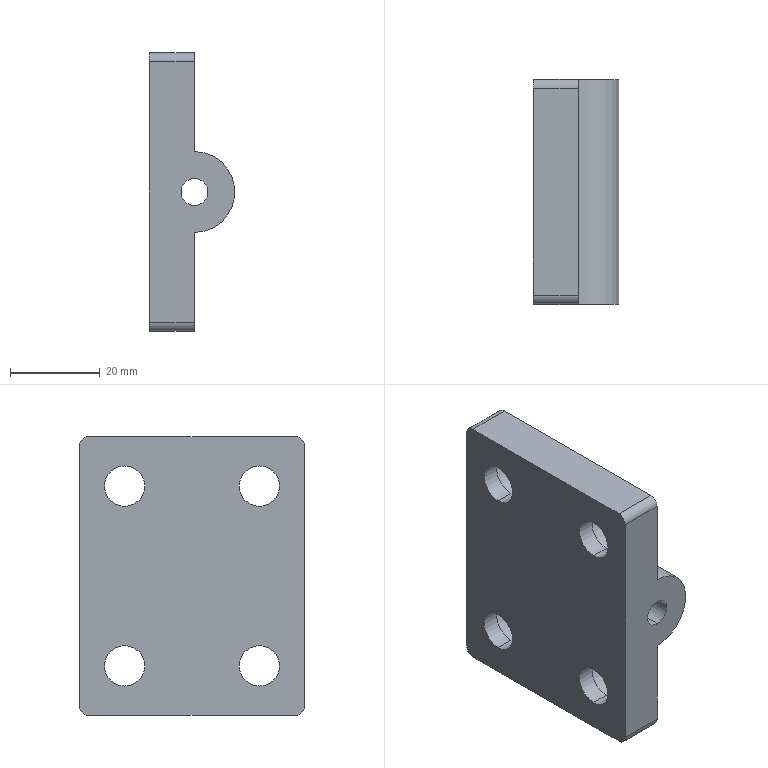Part | SolidWorks | features Extrusion 1, Fillet 1, HoleWzd 1 | 1 solid | 34 faces | box 19 x 50 x 62 mm | volume 31201 mm3 | cylinder 23 | plane 11 | commonest cylinder face diameters 9 x8 14 x8 4 x4 6 x2 18 x1
STEP:
#1=CARTESIAN_POINT('',(4.,15.,27.));
#2=VERTEX_POINT('',#1);
#3=CARTESIAN_POINT('',(4.,15.,13.));
#4=VERTEX_POINT('',#3);
#5=CARTESIAN_POINT('',(4.,15.,20.));
#6=DIRECTION('',(1.,0.,0.));
#7=DIRECTION('',(0.,0.,-1.));
#8=AXIS2_PLACEMENT_3D('',#5,#6,#7);
#9=CIRCLE('',#8,7.);
#10=EDGE_CURVE('',#2,#4,#9,.T.);
#11=ORIENTED_EDGE('',*,*,#10,.F.);
#12=CARTESIAN_POINT('',(10.,15.,27.));
#13=VERTEX_POINT('',#12);
#14=CARTESIAN_POINT('',(10.,15.,27.));
#15=DIRECTION('',(1.,0.,0.));
#16=VECTOR('',#15,1000.);
#17=LINE('',#14,#16);
#18=EDGE_CURVE('',#2,#13,#17,.T.);
#19=ORIENTED_EDGE('',*,*,#18,.T.);
#20=CARTESIAN_POINT('',(10.,15.,13.));
#21=VERTEX_POINT('',#20);
#22=CARTESIAN_POINT('',(10.,15.,20.));
#23=DIRECTION('',(1.,0.,0.));
#24=DIRECTION('',(0.,0.,-1.));
#25=AXIS2_PLACEMENT_3D('',#22,#23,#24);
#26=CIRCLE('',#25,7.);
#27=EDGE_CURVE('',#13,#21,#26,.T.);
#28=ORIENTED_EDGE('',*,*,#27,.T.);
#29=CARTESIAN_POINT('',(10.,15.,13.));
#30=DIRECTION('',(1.,0.,0.));
#31=VECTOR('',#30,1000.);
#32=LINE('',#29,#31);
#33=EDGE_CURVE('',#4,#21,#32,.T.);
#34=ORIENTED_EDGE('',*,*,#33,.F.);
#35=EDGE_LOOP('',(#11,#19,#28,#34));
#36=FACE_OUTER_BOUND('',#35,.T.);
#37=CARTESIAN_POINT('',(10.,15.,20.));
#38=DIRECTION('',(1.,0.,0.));
#39=DIRECTION('',(0.,0.,-1.));
#40=AXIS2_PLACEMENT_3D('',#37,#38,#39);
#41=CYLINDRICAL_SURFACE('',#40,7.);
#42=ADVANCED_FACE('',(#36),#41,.F.);
#43=CARTESIAN_POINT('',(0.,15.,24.5));
#44=VERTEX_POINT('',#43);
#45=CARTESIAN_POINT('',(0.,15.,15.5));
#46=VERTEX_POINT('',#45);
#47=CARTESIAN_POINT('',(0.,15.,20.));
#48=DIRECTION('',(1.,0.,0.));
#49=DIRECTION('',(0.,0.,-1.));
#50=AXIS2_PLACEMENT_3D('',#47,#48,#49);
#51=CIRCLE('',#50,4.5);
#52=EDGE_CURVE('',#44,#46,#51,.T.);
#53=ORIENTED_EDGE('',*,*,#52,.F.);
#54=CARTESIAN_POINT('',(4.,15.,24.5));
#55=VERTEX_POINT('',#54);
#56=CARTESIAN_POINT('',(10.,15.,24.5));
#57=DIRECTION('',(1.,0.,0.));
#58=VECTOR('',#57,1000.);
#59=LINE('',#56,#58);
#60=EDGE_CURVE('',#44,#55,#59,.T.);
#61=ORIENTED_EDGE('',*,*,#60,.T.);
#62=CARTESIAN_POINT('',(4.,15.,15.5));
#63=VERTEX_POINT('',#62);
#64=CARTESIAN_POINT('',(4.,15.,20.));
#65=DIRECTION('',(1.,0.,0.));
#66=DIRECTION('',(0.,0.,-1.));
#67=AXIS2_PLACEMENT_3D('',#64,#65,#66);
#68=CIRCLE('',#67,4.5);
#69=EDGE_CURVE('',#55,#63,#68,.T.);
#70=ORIENTED_EDGE('',*,*,#69,.T.);
#71=CARTESIAN_POINT('',(10.,15.,15.5));
#72=DIRECTION('',(1.,0.,0.));
#73=VECTOR('',#72,1000.);
#74=LINE('',#71,#73);
#75=EDGE_CURVE('',#46,#63,#74,.T.);
#76=ORIENTED_EDGE('',*,*,#75,.F.);
#77=EDGE_LOOP('',(#53,#61,#70,#76));
#78=FACE_OUTER_BOUND('',#77,.T.);
#79=CARTESIAN_POINT('',(10.,15.,20.));
#80=DIRECTION('',(1.,0.,0.));
#81=DIRECTION('',(0.,0.,-1.));
#82=AXIS2_PLACEMENT_3D('',#79,#80,#81);
#83=CYLINDRICAL_SURFACE('',#82,4.5);
#84=ADVANCED_FACE('',(#78),#83,.F.);
#85=CARTESIAN_POINT('',(4.,-15.,27.));
#86=VERTEX_POINT('',#85);
#87=CARTESIAN_POINT('',(4.,-15.,13.));
#88=VERTEX_POINT('',#87);
#89=CARTESIAN_POINT('',(4.,-15.,20.));
#90=DIRECTION('',(1.,0.,0.));
#91=DIRECTION('',(0.,0.,-1.));
#92=AXIS2_PLACEMENT_3D('',#89,#90,#91);
#93=CIRCLE('',#92,7.);
#94=EDGE_CURVE('',#86,#88,#93,.T.);
#95=ORIENTED_EDGE('',*,*,#94,.F.);
#96=CARTESIAN_POINT('',(10.,-15.,27.));
#97=VERTEX_POINT('',#96);
#98=CARTESIAN_POINT('',(10.,-15.,27.));
#99=DIRECTION('',(1.,0.,0.));
#100=VECTOR('',#99,1000.);
#101=LINE('',#98,#100);
#102=EDGE_CURVE('',#86,#97,#101,.T.);
#103=ORIENTED_EDGE('',*,*,#102,.T.);
#104=CARTESIAN_POINT('',(10.,-15.,13.));
#105=VERTEX_POINT('',#104);
#106=CARTESIAN_POINT('',(10.,-15.,20.));
#107=DIRECTION('',(1.,0.,0.));
#108=DIRECTION('',(0.,0.,-1.));
#109=AXIS2_PLACEMENT_3D('',#106,#107,#108);
#110=CIRCLE('',#109,7.);
#111=EDGE_CURVE('',#97,#105,#110,.T.);
#112=ORIENTED_EDGE('',*,*,#111,.T.);
#113=CARTESIAN_POINT('',(10.,-15.,13.));
#114=DIRECTION('',(1.,0.,0.));
#115=VECTOR('',#114,1000.);
#116=LINE('',#113,#115);
#117=EDGE_CURVE('',#88,#105,#116,.T.);
#118=ORIENTED_EDGE('',*,*,#117,.F.);
#119=EDGE_LOOP('',(#95,#103,#112,#118));
#120=FACE_OUTER_BOUND('',#119,.T.);
#121=CARTESIAN_POINT('',(10.,-15.,20.));
#122=DIRECTION('',(1.,0.,0.));
#123=DIRECTION('',(0.,0.,-1.));
#124=AXIS2_PLACEMENT_3D('',#121,#122,#123);
#125=CYLINDRICAL_SURFACE('',#124,7.);
#126=ADVANCED_FACE('',(#120),#125,.F.);
#127=CARTESIAN_POINT('',(0.,-15.,24.5));
#128=VERTEX_POINT('',#127);
#129=CARTESIAN_POINT('',(0.,-15.,15.5));
#130=VERTEX_POINT('',#129);
#131=CARTESIAN_POINT('',(0.,-15.,20.));
#132=DIRECTION('',(1.,0.,0.));
#133=DIRECTION('',(0.,0.,-1.));
#134=AXIS2_PLACEMENT_3D('',#131,#132,#133);
#135=CIRCLE('',#134,4.5);
#136=EDGE_CURVE('',#128,#130,#135,.T.);
#137=ORIENTED_EDGE('',*,*,#136,.F.);
#138=CARTESIAN_POINT('',(4.,-15.,24.5));
#139=VERTEX_POINT('',#138);
#140=CARTESIAN_POINT('',(10.,-15.,24.5));
#141=DIRECTION('',(1.,0.,0.));
#142=VECTOR('',#141,1000.);
#143=LINE('',#140,#142);
#144=EDGE_CURVE('',#128,#139,#143,.T.);
#145=ORIENTED_EDGE('',*,*,#144,.T.);
#146=CARTESIAN_POINT('',(4.,-15.,15.5));
#147=VERTEX_POINT('',#146);
#148=CARTESIAN_POINT('',(4.,-15.,20.));
#149=DIRECTION('',(1.,0.,0.));
#150=DIRECTION('',(0.,0.,-1.));
#151=AXIS2_PLACEMENT_3D('',#148,#149,#150);
#152=CIRCLE('',#151,4.5);
#153=EDGE_CURVE('',#139,#147,#152,.T.);
#154=ORIENTED_EDGE('',*,*,#153,.T.);
#155=CARTESIAN_POINT('',(10.,-15.,15.5));
#156=DIRECTION('',(1.,0.,0.));
#157=VECTOR('',#156,1000.);
#158=LINE('',#155,#157);
#159=EDGE_CURVE('',#130,#147,#158,.T.);
#160=ORIENTED_EDGE('',*,*,#159,.F.);
#161=EDGE_LOOP('',(#137,#145,#154,#160));
#162=FACE_OUTER_BOUND('',#161,.T.);
#163=CARTESIAN_POINT('',(10.,-15.,20.));
#164=DIRECTION('',(1.,0.,0.));
#165=DIRECTION('',(0.,0.,-1.));
#166=AXIS2_PLACEMENT_3D('',#163,#164,#165);
#167=CYLINDRICAL_SURFACE('',#166,4.5);
#168=ADVANCED_FACE('',(#162),#167,.F.);
#169=CARTESIAN_POINT('',(4.,-15.,-13.));
#170=VERTEX_POINT('',#169);
#171=CARTESIAN_POINT('',(4.,-15.,-27.));
#172=VERTEX_POINT('',#171);
#173=CARTESIAN_POINT('',(4.,-15.,-20.));
#174=DIRECTION('',(1.,0.,0.));
#175=DIRECTION('',(0.,0.,-1.));
#176=AXIS2_PLACEMENT_3D('',#173,#174,#175);
#177=CIRCLE('',#176,7.);
#178=EDGE_CURVE('',#170,#172,#177,.T.);
#179=ORIENTED_EDGE('',*,*,#178,.F.);
#180=CARTESIAN_POINT('',(10.,-15.,-13.));
#181=VERTEX_POINT('',#180);
#182=CARTESIAN_POINT('',(10.,-15.,-13.));
#183=DIRECTION('',(1.,0.,0.));
#184=VECTOR('',#183,1000.);
#185=LINE('',#182,#184);
#186=EDGE_CURVE('',#170,#181,#185,.T.);
#187=ORIENTED_EDGE('',*,*,#186,.T.);
#188=CARTESIAN_POINT('',(10.,-15.,-27.));
#189=VERTEX_POINT('',#188);
#190=CARTESIAN_POINT('',(10.,-15.,-20.));
#191=DIRECTION('',(1.,0.,0.));
#192=DIRECTION('',(0.,0.,-1.));
#193=AXIS2_PLACEMENT_3D('',#190,#191,#192);
#194=CIRCLE('',#193,7.);
#195=EDGE_CURVE('',#181,#189,#194,.T.);
#196=ORIENTED_EDGE('',*,*,#195,.T.);
#197=CARTESIAN_POINT('',(10.,-15.,-27.));
#198=DIRECTION('',(1.,0.,0.));
#199=VECTOR('',#198,1000.);
#200=LINE('',#197,#199);
#201=EDGE_CURVE('',#172,#189,#200,.T.);
#202=ORIENTED_EDGE('',*,*,#201,.F.);
#203=EDGE_LOOP('',(#179,#187,#196,#202));
#204=FACE_OUTER_BOUND('',#203,.T.);
#205=CARTESIAN_POINT('',(10.,-15.,-20.));
#206=DIRECTION('',(1.,0.,0.));
#207=DIRECTION('',(0.,0.,-1.));
#208=AXIS2_PLACEMENT_3D('',#205,#206,#207);
#209=CYLINDRICAL_SURFACE('',#208,7.);
#210=ADVANCED_FACE('',(#204),#209,.F.);
#211=CARTESIAN_POINT('',(0.,-15.,-15.5));
#212=VERTEX_POINT('',#211);
#213=CARTESIAN_POINT('',(0.,-15.,-24.5));
#214=VERTEX_POINT('',#213);
#215=CARTESIAN_POINT('',(0.,-15.,-20.));
#216=DIRECTION('',(1.,0.,0.));
#217=DIRECTION('',(0.,0.,-1.));
#218=AXIS2_PLACEMENT_3D('',#215,#216,#217);
#219=CIRCLE('',#218,4.5);
#220=EDGE_CURVE('',#212,#214,#219,.T.);
#221=ORIENTED_EDGE('',*,*,#220,.F.);
#222=CARTESIAN_POINT('',(4.,-15.,-15.5));
#223=VERTEX_POINT('',#222);
#224=CARTESIAN_POINT('',(10.,-15.,-15.5));
#225=DIRECTION('',(1.,0.,0.));
#226=VECTOR('',#225,1000.);
#227=LINE('',#224,#226);
#228=EDGE_CURVE('',#212,#223,#227,.T.);
#229=ORIENTED_EDGE('',*,*,#228,.T.);
#230=CARTESIAN_POINT('',(4.,-15.,-24.5));
#231=VERTEX_POINT('',#230);
#232=CARTESIAN_POINT('',(4.,-15.,-20.));
#233=DIRECTION('',(1.,0.,0.));
#234=DIRECTION('',(0.,0.,-1.));
#235=AXIS2_PLACEMENT_3D('',#232,#233,#234);
#236=CIRCLE('',#235,4.5);
#237=EDGE_CURVE('',#223,#231,#236,.T.);
#238=ORIENTED_EDGE('',*,*,#237,.T.);
#239=CARTESIAN_POINT('',(10.,-15.,-24.5));
#240=DIRECTION('',(1.,0.,0.));
#241=VECTOR('',#240,1000.);
#242=LINE('',#239,#241);
#243=EDGE_CURVE('',#214,#231,#242,.T.);
#244=ORIENTED_EDGE('',*,*,#243,.F.);
#245=EDGE_LOOP('',(#221,#229,#238,#244));
#246=FACE_OUTER_BOUND('',#245,.T.);
#247=CARTESIAN_POINT('',(10.,-15.,-20.));
#248=DIRECTION('',(1.,0.,0.));
#249=DIRECTION('',(0.,0.,-1.));
#250=AXIS2_PLACEMENT_3D('',#247,#248,#249);
#251=CYLINDRICAL_SURFACE('',#250,4.5);
#252=ADVANCED_FACE('',(#246),#251,.F.);
#253=CARTESIAN_POINT('',(4.,15.,-13.));
#254=VERTEX_POINT('',#253);
#255=CARTESIAN_POINT('',(4.,15.,-27.));
#256=VERTEX_POINT('',#255);
#257=CARTESIAN_POINT('',(4.,15.,-20.));
#258=DIRECTION('',(1.,0.,0.));
#259=DIRECTION('',(0.,0.,-1.));
#260=AXIS2_PLACEMENT_3D('',#257,#258,#259);
#261=CIRCLE('',#260,7.);
#262=EDGE_CURVE('',#254,#256,#261,.T.);
#263=ORIENTED_EDGE('',*,*,#262,.F.);
#264=CARTESIAN_POINT('',(10.,15.,-13.));
#265=VERTEX_POINT('',#264);
#266=CARTESIAN_POINT('',(10.,15.,-13.));
#267=DIRECTION('',(1.,0.,0.));
#268=VECTOR('',#267,1000.);
#269=LINE('',#266,#268);
#270=EDGE_CURVE('',#254,#265,#269,.T.);
#271=ORIENTED_EDGE('',*,*,#270,.T.);
#272=CARTESIAN_POINT('',(10.,15.,-27.));
#273=VERTEX_POINT('',#272);
#274=CARTESIAN_POINT('',(10.,15.,-20.));
#275=DIRECTION('',(1.,0.,0.));
#276=DIRECTION('',(0.,0.,-1.));
#277=AXIS2_PLACEMENT_3D('',#274,#275,#276);
#278=CIRCLE('',#277,7.);
#279=EDGE_CURVE('',#265,#273,#278,.T.);
#280=ORIENTED_EDGE('',*,*,#279,.T.);
#281=CARTESIAN_POINT('',(10.,15.,-27.));
#282=DIRECTION('',(1.,0.,0.));
#283=VECTOR('',#282,1000.);
#284=LINE('',#281,#283);
#285=EDGE_CURVE('',#256,#273,#284,.T.);
#286=ORIENTED_EDGE('',*,*,#285,.F.);
#287=EDGE_LOOP('',(#263,#271,#280,#286));
#288=FACE_OUTER_BOUND('',#287,.T.);
#289=CARTESIAN_POINT('',(10.,15.,-20.));
#290=DIRECTION('',(1.,0.,0.));
#291=DIRECTION('',(0.,0.,-1.));
#292=AXIS2_PLACEMENT_3D('',#289,#290,#291);
#293=CYLINDRICAL_SURFACE('',#292,7.);
#294=ADVANCED_FACE('',(#288),#293,.F.);
#295=CARTESIAN_POINT('',(0.,15.,-15.5));
#296=VERTEX_POINT('',#295);
#297=CARTESIAN_POINT('',(0.,15.,-24.5));
#298=VERTEX_POINT('',#297);
#299=CARTESIAN_POINT('',(0.,15.,-20.));
#300=DIRECTION('',(1.,0.,0.));
#301=DIRECTION('',(0.,0.,-1.));
#302=AXIS2_PLACEMENT_3D('',#299,#300,#301);
#303=CIRCLE('',#302,4.5);
#304=EDGE_CURVE('',#296,#298,#303,.T.);
#305=ORIENTED_EDGE('',*,*,#304,.F.);
#306=CARTESIAN_POINT('',(4.,15.,-15.5));
#307=VERTEX_POINT('',#306);
#308=CARTESIAN_POINT('',(10.,15.,-15.5));
#309=DIRECTION('',(1.,0.,0.));
#310=VECTOR('',#309,1000.);
#311=LINE('',#308,#310);
#312=EDGE_CURVE('',#296,#307,#311,.T.);
#313=ORIENTED_EDGE('',*,*,#312,.T.);
#314=CARTESIAN_POINT('',(4.,15.,-24.5));
#315=VERTEX_POINT('',#314);
#316=CARTESIAN_POINT('',(4.,15.,-20.));
#317=DIRECTION('',(1.,0.,0.));
#318=DIRECTION('',(0.,0.,-1.));
#319=AXIS2_PLACEMENT_3D('',#316,#317,#318);
#320=CIRCLE('',#319,4.5);
#321=EDGE_CURVE('',#307,#315,#320,.T.);
#322=ORIENTED_EDGE('',*,*,#321,.T.);
#323=CARTESIAN_POINT('',(10.,15.,-24.5));
#324=DIRECTION('',(1.,0.,0.));
#325=VECTOR('',#324,1000.);
#326=LINE('',#323,#325);
#327=EDGE_CURVE('',#298,#315,#326,.T.);
#328=ORIENTED_EDGE('',*,*,#327,.F.);
#329=EDGE_LOOP('',(#305,#313,#322,#328));
#330=FACE_OUTER_BOUND('',#329,.T.);
#331=CARTESIAN_POINT('',(10.,15.,-20.));
#332=DIRECTION('',(1.,0.,0.));
#333=DIRECTION('',(0.,0.,-1.));
#334=AXIS2_PLACEMENT_3D('',#331,#332,#333);
#335=CYLINDRICAL_SURFACE('',#334,4.5);
#336=ADVANCED_FACE('',(#330),#335,.F.);
#337=CARTESIAN_POINT('',(10.,25.,-3.));
#338=VERTEX_POINT('',#337);
#339=CARTESIAN_POINT('',(10.,25.,3.));
#340=VERTEX_POINT('',#339);
#341=CARTESIAN_POINT('',(10.,25.,0.));
#342=DIRECTION('',(0.,1.,0.));
#343=DIRECTION('',(0.,0.,1.));
#344=AXIS2_PLACEMENT_3D('',#341,#342,#343);
#345=CIRCLE('',#344,3.);
#346=EDGE_CURVE('',#338,#340,#345,.T.);
#347=ORIENTED_EDGE('',*,*,#346,.T.);
#348=CARTESIAN_POINT('',(10.,-25.,3.));
#349=VERTEX_POINT('',#348);
#350=CARTESIAN_POINT('',(10.,25.,3.));
#351=DIRECTION('',(0.,-1.,0.));
#352=VECTOR('',#351,1000.);
#353=LINE('',#350,#352);
#354=EDGE_CURVE('',#340,#349,#353,.T.);
#355=ORIENTED_EDGE('',*,*,#354,.T.);
#356=CARTESIAN_POINT('',(10.,-25.,-3.));
#357=VERTEX_POINT('',#356);
#358=CARTESIAN_POINT('',(10.,-25.,0.));
#359=DIRECTION('',(0.,1.,0.));
#360=DIRECTION('',(0.,0.,1.));
#361=AXIS2_PLACEMENT_3D('',#358,#359,#360);
#362=CIRCLE('',#361,3.);
#363=EDGE_CURVE('',#357,#349,#362,.T.);
#364=ORIENTED_EDGE('',*,*,#363,.F.);
#365=CARTESIAN_POINT('',(10.,25.,-3.));
#366=DIRECTION('',(0.,-1.,0.));
#367=VECTOR('',#366,1000.);
#368=LINE('',#365,#367);
#369=EDGE_CURVE('',#338,#357,#368,.T.);
#370=ORIENTED_EDGE('',*,*,#369,.F.);
#371=EDGE_LOOP('',(#347,#355,#364,#370));
#372=FACE_OUTER_BOUND('',#371,.T.);
#373=CARTESIAN_POINT('',(10.,25.,0.));
#374=DIRECTION('',(0.,-1.,0.));
#375=DIRECTION('',(0.,0.,-1.));
#376=AXIS2_PLACEMENT_3D('',#373,#374,#375);
#377=CYLINDRICAL_SURFACE('',#376,3.);
#378=ADVANCED_FACE('',(#372),#377,.F.);
#379=CARTESIAN_POINT('',(10.,25.,-9.));
#380=VERTEX_POINT('',#379);
#381=CARTESIAN_POINT('',(10.,25.,-29.));
#382=VERTEX_POINT('',#381);
#383=CARTESIAN_POINT('',(10.,25.,-31.));
#384=DIRECTION('',(0.,0.,-1.));
#385=VECTOR('',#384,1000.);
#386=LINE('',#383,#385);
#387=EDGE_CURVE('',#380,#382,#386,.T.);
#388=ORIENTED_EDGE('',*,*,#387,.T.);
#389=CARTESIAN_POINT('',(0.,25.,-29.));
#390=VERTEX_POINT('',#389);
#391=CARTESIAN_POINT('',(0.,25.,-29.));
#392=DIRECTION('',(-1.,0.,0.));
#393=VECTOR('',#392,1000.);
#394=LINE('',#391,#393);
#395=EDGE_CURVE('',#382,#390,#394,.T.);
#396=ORIENTED_EDGE('',*,*,#395,.T.);
#397=CARTESIAN_POINT('',(0.,25.,29.));
#398=VERTEX_POINT('',#397);
#399=CARTESIAN_POINT('',(0.,25.,-31.));
#400=DIRECTION('',(0.,0.,1.));
#401=VECTOR('',#400,1000.);
#402=LINE('',#399,#401);
#403=EDGE_CURVE('',#390,#398,#402,.T.);
#404=ORIENTED_EDGE('',*,*,#403,.T.);
#405=CARTESIAN_POINT('',(10.,25.,29.));
#406=VERTEX_POINT('',#405);
#407=CARTESIAN_POINT('',(10.,25.,29.));
#408=DIRECTION('',(1.,0.,0.));
#409=VECTOR('',#408,1000.);
#410=LINE('',#407,#409);
#411=EDGE_CURVE('',#398,#406,#410,.T.);
#412=ORIENTED_EDGE('',*,*,#411,.T.);
#413=CARTESIAN_POINT('',(10.,25.,9.));
#414=VERTEX_POINT('',#413);
#415=CARTESIAN_POINT('',(10.,25.,9.));
#416=DIRECTION('',(0.,0.,-1.));
#417=VECTOR('',#416,1000.);
#418=LINE('',#415,#417);
#419=EDGE_CURVE('',#406,#414,#418,.T.);
#420=ORIENTED_EDGE('',*,*,#419,.T.);
#421=CARTESIAN_POINT('',(10.,25.,0.));
#422=DIRECTION('',(0.,1.,0.));
#423=DIRECTION('',(0.,0.,1.));
#424=AXIS2_PLACEMENT_3D('',#421,#422,#423);
#425=CIRCLE('',#424,9.);
#426=EDGE_CURVE('',#414,#380,#425,.T.);
#427=ORIENTED_EDGE('',*,*,#426,.T.);
#428=EDGE_LOOP('',(#388,#396,#404,#412,#420,#427));
#429=FACE_OUTER_BOUND('',#428,.T.);
#430=ORIENTED_EDGE('',*,*,#346,.F.);
#431=CARTESIAN_POINT('',(10.,25.,0.));
#432=DIRECTION('',(0.,1.,0.));
#433=DIRECTION('',(0.,0.,1.));
#434=AXIS2_PLACEMENT_3D('',#431,#432,#433);
#435=CIRCLE('',#434,3.);
#436=EDGE_CURVE('',#340,#338,#435,.T.);
#437=ORIENTED_EDGE('',*,*,#436,.F.);
#438=EDGE_LOOP('',(#430,#437));
#439=FACE_BOUND('',#438,.T.);
#440=CARTESIAN_POINT('',(10.,25.,0.));
#441=DIRECTION('',(0.,1.,0.));
#442=DIRECTION('',(0.,0.,1.));
#443=AXIS2_PLACEMENT_3D('',#440,#441,#442);
#444=PLANE('',#443);
#445=ADVANCED_FACE('',(#429,#439),#444,.T.);
#446=CARTESIAN_POINT('',(10.,-25.,29.));
#447=VERTEX_POINT('',#446);
#448=CARTESIAN_POINT('',(10.,-25.,9.));
#449=VERTEX_POINT('',#448);
#450=CARTESIAN_POINT('',(10.,-25.,9.));
#451=DIRECTION('',(0.,0.,-1.));
#452=VECTOR('',#451,1000.);
#453=LINE('',#450,#452);
#454=EDGE_CURVE('',#447,#449,#453,.T.);
#455=ORIENTED_EDGE('',*,*,#454,.F.);
#456=CARTESIAN_POINT('',(0.,-25.,29.));
#457=VERTEX_POINT('',#456);
#458=CARTESIAN_POINT('',(10.,-25.,29.));
#459=DIRECTION('',(-1.,0.,0.));
#460=VECTOR('',#459,1000.);
#461=LINE('',#458,#460);
#462=EDGE_CURVE('',#447,#457,#461,.T.);
#463=ORIENTED_EDGE('',*,*,#462,.T.);
#464=CARTESIAN_POINT('',(0.,-25.,-29.));
#465=VERTEX_POINT('',#464);
#466=CARTESIAN_POINT('',(0.,-25.,-31.));
#467=DIRECTION('',(0.,0.,1.));
#468=VECTOR('',#467,1000.);
#469=LINE('',#466,#468);
#470=EDGE_CURVE('',#465,#457,#469,.T.);
#471=ORIENTED_EDGE('',*,*,#470,.F.);
#472=CARTESIAN_POINT('',(10.,-25.,-29.));
#473=VERTEX_POINT('',#472);
#474=CARTESIAN_POINT('',(10.,-25.,-29.));
#475=DIRECTION('',(1.,0.,0.));
#476=VECTOR('',#475,1000.);
#477=LINE('',#474,#476);
#478=EDGE_CURVE('',#465,#473,#477,.T.);
#479=ORIENTED_EDGE('',*,*,#478,.T.);
#480=CARTESIAN_POINT('',(10.,-25.,-9.));
#481=VERTEX_POINT('',#480);
#482=CARTESIAN_POINT('',(10.,-25.,-31.));
#483=DIRECTION('',(0.,0.,-1.));
#484=VECTOR('',#483,1000.);
#485=LINE('',#482,#484);
#486=EDGE_CURVE('',#481,#473,#485,.T.);
#487=ORIENTED_EDGE('',*,*,#486,.F.);
#488=CARTESIAN_POINT('',(10.,-25.,0.));
#489=DIRECTION('',(0.,1.,0.));
#490=DIRECTION('',(0.,0.,1.));
#491=AXIS2_PLACEMENT_3D('',#488,#489,#490);
#492=CIRCLE('',#491,9.);
#493=EDGE_CURVE('',#449,#481,#492,.T.);
#494=ORIENTED_EDGE('',*,*,#493,.F.);
#495=EDGE_LOOP('',(#455,#463,#471,#479,#487,#494));
#496=FACE_OUTER_BOUND('',#495,.T.);
#497=ORIENTED_EDGE('',*,*,#363,.T.);
#498=CARTESIAN_POINT('',(10.,-25.,0.));
#499=DIRECTION('',(0.,1.,0.));
#500=DIRECTION('',(0.,0.,1.));
#501=AXIS2_PLACEMENT_3D('',#498,#499,#500);
#502=CIRCLE('',#501,3.);
#503=EDGE_CURVE('',#349,#357,#502,.T.);
#504=ORIENTED_EDGE('',*,*,#503,.T.);
#505=EDGE_LOOP('',(#497,#504));
#506=FACE_BOUND('',#505,.T.);
#507=CARTESIAN_POINT('',(10.,-25.,0.));
#508=DIRECTION('',(0.,1.,0.));
#509=DIRECTION('',(0.,0.,1.));
#510=AXIS2_PLACEMENT_3D('',#507,#508,#509);
#511=PLANE('',#510);
#512=ADVANCED_FACE('',(#496,#506),#511,.F.);
#513=CARTESIAN_POINT('',(0.,15.,20.));
#514=DIRECTION('',(1.,0.,0.));
#515=DIRECTION('',(0.,0.,-1.));
#516=AXIS2_PLACEMENT_3D('',#513,#514,#515);
#517=CIRCLE('',#516,4.5);
#518=EDGE_CURVE('',#46,#44,#517,.T.);
#519=ORIENTED_EDGE('',*,*,#518,.T.);
#520=ORIENTED_EDGE('',*,*,#52,.T.);
#521=EDGE_LOOP('',(#519,#520));
#522=FACE_BOUND('',#521,.T.);
#523=CARTESIAN_POINT('',(0.,-15.,20.));
#524=DIRECTION('',(1.,0.,0.));
#525=DIRECTION('',(0.,0.,-1.));
#526=AXIS2_PLACEMENT_3D('',#523,#524,#525);
#527=CIRCLE('',#526,4.5);
#528=EDGE_CURVE('',#130,#128,#527,.T.);
#529=ORIENTED_EDGE('',*,*,#528,.T.);
#530=ORIENTED_EDGE('',*,*,#136,.T.);
#531=EDGE_LOOP('',(#529,#530));
#532=FACE_BOUND('',#531,.T.);
#533=CARTESIAN_POINT('',(0.,-15.,-20.));
#534=DIRECTION('',(1.,0.,0.));
#535=DIRECTION('',(0.,0.,-1.));
#536=AXIS2_PLACEMENT_3D('',#533,#534,#535);
#537=CIRCLE('',#536,4.5);
#538=EDGE_CURVE('',#214,#212,#537,.T.);
#539=ORIENTED_EDGE('',*,*,#538,.T.);
#540=ORIENTED_EDGE('',*,*,#220,.T.);
#541=EDGE_LOOP('',(#539,#540));
#542=FACE_BOUND('',#541,.T.);
#543=CARTESIAN_POINT('',(0.,15.,-20.));
#544=DIRECTION('',(1.,0.,0.));
#545=DIRECTION('',(0.,0.,-1.));
#546=AXIS2_PLACEMENT_3D('',#543,#544,#545);
#547=CIRCLE('',#546,4.5);
#548=EDGE_CURVE('',#298,#296,#547,.T.);
#549=ORIENTED_EDGE('',*,*,#548,.T.);
#550=ORIENTED_EDGE('',*,*,#304,.T.);
#551=EDGE_LOOP('',(#549,#550));
#552=FACE_BOUND('',#551,.T.);
#553=ORIENTED_EDGE('',*,*,#470,.T.);
#554=CARTESIAN_POINT('',(0.,-23.,31.));
#555=VERTEX_POINT('',#554);
#556=CARTESIAN_POINT('',(0.,-23.,29.));
#557=DIRECTION('',(-1.,0.,0.));
#558=DIRECTION('',(0.,0.,-1.));
#559=AXIS2_PLACEMENT_3D('',#556,#557,#558);
#560=CIRCLE('',#559,2.);
#561=EDGE_CURVE('',#457,#555,#560,.T.);
#562=ORIENTED_EDGE('',*,*,#561,.T.);
#563=CARTESIAN_POINT('',(0.,23.,31.));
#564=VERTEX_POINT('',#563);
#565=CARTESIAN_POINT('',(0.,25.,31.));
#566=DIRECTION('',(0.,-1.,0.));
#567=VECTOR('',#566,1000.);
#568=LINE('',#565,#567);
#569=EDGE_CURVE('',#564,#555,#568,.T.);
#570=ORIENTED_EDGE('',*,*,#569,.F.);
#571=CARTESIAN_POINT('',(0.,23.,29.));
#572=DIRECTION('',(-1.,0.,0.));
#573=DIRECTION('',(0.,0.,-1.));
#574=AXIS2_PLACEMENT_3D('',#571,#572,#573);
#575=CIRCLE('',#574,2.);
#576=EDGE_CURVE('',#564,#398,#575,.T.);
#577=ORIENTED_EDGE('',*,*,#576,.T.);
#578=ORIENTED_EDGE('',*,*,#403,.F.);
#579=CARTESIAN_POINT('',(0.,23.,-31.));
#580=VERTEX_POINT('',#579);
#581=CARTESIAN_POINT('',(0.,23.,-29.));
#582=DIRECTION('',(-1.,0.,0.));
#583=DIRECTION('',(0.,0.,-1.));
#584=AXIS2_PLACEMENT_3D('',#581,#582,#583);
#585=CIRCLE('',#584,2.);
#586=EDGE_CURVE('',#390,#580,#585,.T.);
#587=ORIENTED_EDGE('',*,*,#586,.T.);
#588=CARTESIAN_POINT('',(0.,-23.,-31.));
#589=VERTEX_POINT('',#588);
#590=CARTESIAN_POINT('',(0.,25.,-31.));
#591=DIRECTION('',(0.,-1.,0.));
#592=VECTOR('',#591,1000.);
#593=LINE('',#590,#592);
#594=EDGE_CURVE('',#580,#589,#593,.T.);
#595=ORIENTED_EDGE('',*,*,#594,.T.);
#596=CARTESIAN_POINT('',(0.,-23.,-29.));
#597=DIRECTION('',(-1.,0.,0.));
#598=DIRECTION('',(0.,0.,-1.));
#599=AXIS2_PLACEMENT_3D('',#596,#597,#598);
#600=CIRCLE('',#599,2.);
#601=EDGE_CURVE('',#589,#465,#600,.T.);
#602=ORIENTED_EDGE('',*,*,#601,.T.);
#603=EDGE_LOOP('',(#553,#562,#570,#577,#578,#587,#595,#602));
#604=FACE_OUTER_BOUND('',#603,.T.);
#605=CARTESIAN_POINT('',(0.,25.,-31.));
#606=DIRECTION('',(1.,0.,0.));
#607=DIRECTION('',(0.,0.,-1.));
#608=AXIS2_PLACEMENT_3D('',#605,#606,#607);
#609=PLANE('',#608);
#610=ADVANCED_FACE('',(#522,#532,#542,#552,#604),#609,.F.);
#611=ORIENTED_EDGE('',*,*,#569,.T.);
#612=CARTESIAN_POINT('',(10.,-23.,31.));
#613=VERTEX_POINT('',#612);
#614=CARTESIAN_POINT('',(0.,-23.,31.));
#615=DIRECTION('',(1.,0.,0.));
#616=VECTOR('',#615,1000.);
#617=LINE('',#614,#616);
#618=EDGE_CURVE('',#555,#613,#617,.T.);
#619=ORIENTED_EDGE('',*,*,#618,.T.);
#620=CARTESIAN_POINT('',(10.,23.,31.));
#621=VERTEX_POINT('',#620);
#622=CARTESIAN_POINT('',(10.,25.,31.));
#623=DIRECTION('',(0.,-1.,0.));
#624=VECTOR('',#623,1000.);
#625=LINE('',#622,#624);
#626=EDGE_CURVE('',#621,#613,#625,.T.);
#627=ORIENTED_EDGE('',*,*,#626,.F.);
#628=CARTESIAN_POINT('',(0.,23.,31.));
#629=DIRECTION('',(-1.,0.,0.));
#630=VECTOR('',#629,1000.);
#631=LINE('',#628,#630);
#632=EDGE_CURVE('',#621,#564,#631,.T.);
#633=ORIENTED_EDGE('',*,*,#632,.T.);
#634=EDGE_LOOP('',(#611,#619,#627,#633));
#635=FACE_OUTER_BOUND('',#634,.T.);
#636=CARTESIAN_POINT('',(0.,25.,31.));
#637=DIRECTION('',(0.,0.,-1.));
#638=DIRECTION('',(-1.,0.,0.));
#639=AXIS2_PLACEMENT_3D('',#636,#637,#638);
#640=PLANE('',#639);
#641=ADVANCED_FACE('',(#635),#640,.F.);
#642=CARTESIAN_POINT('',(10.,15.,20.));
#643=DIRECTION('',(1.,0.,0.));
#644=DIRECTION('',(0.,0.,-1.));
#645=AXIS2_PLACEMENT_3D('',#642,#643,#644);
#646=CIRCLE('',#645,7.);
#647=EDGE_CURVE('',#21,#13,#646,.T.);
#648=ORIENTED_EDGE('',*,*,#647,.F.);
#649=ORIENTED_EDGE('',*,*,#27,.F.);
#650=EDGE_LOOP('',(#648,#649));
#651=FACE_BOUND('',#650,.T.);
#652=CARTESIAN_POINT('',(10.,-15.,20.));
#653=DIRECTION('',(1.,0.,0.));
#654=DIRECTION('',(0.,0.,-1.));
#655=AXIS2_PLACEMENT_3D('',#652,#653,#654);
#656=CIRCLE('',#655,7.);
#657=EDGE_CURVE('',#105,#97,#656,.T.);
#658=ORIENTED_EDGE('',*,*,#657,.F.);
#659=ORIENTED_EDGE('',*,*,#111,.F.);
#660=EDGE_LOOP('',(#658,#659));
#661=FACE_BOUND('',#660,.T.);
#662=ORIENTED_EDGE('',*,*,#626,.T.);
#663=CARTESIAN_POINT('',(10.,-23.,29.));
#664=DIRECTION('',(1.,0.,0.));
#665=DIRECTION('',(0.,0.,1.));
#666=AXIS2_PLACEMENT_3D('',#663,#664,#665);
#667=CIRCLE('',#666,2.);
#668=EDGE_CURVE('',#613,#447,#667,.T.);
#669=ORIENTED_EDGE('',*,*,#668,.T.);
#670=ORIENTED_EDGE('',*,*,#454,.T.);
#671=CARTESIAN_POINT('',(10.,25.,9.));
#672=DIRECTION('',(0.,-1.,0.));
#673=VECTOR('',#672,1000.);
#674=LINE('',#671,#673);
#675=EDGE_CURVE('',#414,#449,#674,.T.);
#676=ORIENTED_EDGE('',*,*,#675,.F.);
#677=ORIENTED_EDGE('',*,*,#419,.F.);
#678=CARTESIAN_POINT('',(10.,23.,29.));
#679=DIRECTION('',(1.,0.,0.));
#680=DIRECTION('',(0.,0.,1.));
#681=AXIS2_PLACEMENT_3D('',#678,#679,#680);
#682=CIRCLE('',#681,2.);
#683=EDGE_CURVE('',#406,#621,#682,.T.);
#684=ORIENTED_EDGE('',*,*,#683,.T.);
#685=EDGE_LOOP('',(#662,#669,#670,#676,#677,#684));
#686=FACE_OUTER_BOUND('',#685,.T.);
#687=CARTESIAN_POINT('',(10.,25.,9.));
#688=DIRECTION('',(-1.,0.,0.));
#689=DIRECTION('',(0.,0.,1.));
#690=AXIS2_PLACEMENT_3D('',#687,#688,#689);
#691=PLANE('',#690);
#692=ADVANCED_FACE('',(#651,#661,#686),#691,.F.);
#693=ORIENTED_EDGE('',*,*,#493,.T.);
#694=CARTESIAN_POINT('',(10.,25.,-9.));
#695=DIRECTION('',(0.,-1.,0.));
#696=VECTOR('',#695,1000.);
#697=LINE('',#694,#696);
#698=EDGE_CURVE('',#380,#481,#697,.T.);
#699=ORIENTED_EDGE('',*,*,#698,.F.);
#700=ORIENTED_EDGE('',*,*,#426,.F.);
#701=ORIENTED_EDGE('',*,*,#675,.T.);
#702=EDGE_LOOP('',(#693,#699,#700,#701));
#703=FACE_OUTER_BOUND('',#702,.T.);
#704=CARTESIAN_POINT('',(10.,25.,0.));
#705=DIRECTION('',(0.,-1.,0.));
#706=DIRECTION('',(0.,0.,-1.));
#707=AXIS2_PLACEMENT_3D('',#704,#705,#706);
#708=CYLINDRICAL_SURFACE('',#707,9.);
#709=ADVANCED_FACE('',(#703),#708,.T.);
#710=CARTESIAN_POINT('',(10.,-15.,-20.));
#711=DIRECTION('',(1.,0.,0.));
#712=DIRECTION('',(0.,0.,-1.));
#713=AXIS2_PLACEMENT_3D('',#710,#711,#712);
#714=CIRCLE('',#713,7.);
#715=EDGE_CURVE('',#189,#181,#714,.T.);
#716=ORIENTED_EDGE('',*,*,#715,.F.);
#717=ORIENTED_EDGE('',*,*,#195,.F.);
#718=EDGE_LOOP('',(#716,#717));
#719=FACE_BOUND('',#718,.T.);
#720=CARTESIAN_POINT('',(10.,15.,-20.));
#721=DIRECTION('',(1.,0.,0.));
#722=DIRECTION('',(0.,0.,-1.));
#723=AXIS2_PLACEMENT_3D('',#720,#721,#722);
#724=CIRCLE('',#723,7.);
#725=EDGE_CURVE('',#273,#265,#724,.T.);
#726=ORIENTED_EDGE('',*,*,#725,.F.);
#727=ORIENTED_EDGE('',*,*,#279,.F.);
#728=EDGE_LOOP('',(#726,#727));
#729=FACE_BOUND('',#728,.T.);
#730=ORIENTED_EDGE('',*,*,#486,.T.);
#731=CARTESIAN_POINT('',(10.,-23.,-31.));
#732=VERTEX_POINT('',#731);
#733=CARTESIAN_POINT('',(10.,-23.,-29.));
#734=DIRECTION('',(1.,0.,0.));
#735=DIRECTION('',(0.,0.,1.));
#736=AXIS2_PLACEMENT_3D('',#733,#734,#735);
#737=CIRCLE('',#736,2.);
#738=EDGE_CURVE('',#473,#732,#737,.T.);
#739=ORIENTED_EDGE('',*,*,#738,.T.);
#740=CARTESIAN_POINT('',(10.,23.,-31.));
#741=VERTEX_POINT('',#740);
#742=CARTESIAN_POINT('',(10.,25.,-31.));
#743=DIRECTION('',(0.,-1.,0.));
#744=VECTOR('',#743,1000.);
#745=LINE('',#742,#744);
#746=EDGE_CURVE('',#741,#732,#745,.T.);
#747=ORIENTED_EDGE('',*,*,#746,.F.);
#748=CARTESIAN_POINT('',(10.,23.,-29.));
#749=DIRECTION('',(1.,0.,0.));
#750=DIRECTION('',(0.,0.,1.));
#751=AXIS2_PLACEMENT_3D('',#748,#749,#750);
#752=CIRCLE('',#751,2.);
#753=EDGE_CURVE('',#741,#382,#752,.T.);
#754=ORIENTED_EDGE('',*,*,#753,.T.);
#755=ORIENTED_EDGE('',*,*,#387,.F.);
#756=ORIENTED_EDGE('',*,*,#698,.T.);
#757=EDGE_LOOP('',(#730,#739,#747,#754,#755,#756));
#758=FACE_OUTER_BOUND('',#757,.T.);
#759=CARTESIAN_POINT('',(10.,25.,-31.));
#760=DIRECTION('',(-1.,0.,0.));
#761=DIRECTION('',(0.,0.,1.));
#762=AXIS2_PLACEMENT_3D('',#759,#760,#761);
#763=PLANE('',#762);
#764=ADVANCED_FACE('',(#719,#729,#758),#763,.F.);
#765=ORIENTED_EDGE('',*,*,#746,.T.);
#766=CARTESIAN_POINT('',(0.,-23.,-31.));
#767=DIRECTION('',(-1.,0.,0.));
#768=VECTOR('',#767,1000.);
#769=LINE('',#766,#768);
#770=EDGE_CURVE('',#732,#589,#769,.T.);
#771=ORIENTED_EDGE('',*,*,#770,.T.);
#772=ORIENTED_EDGE('',*,*,#594,.F.);
#773=CARTESIAN_POINT('',(10.,23.,-31.));
#774=DIRECTION('',(1.,0.,0.));
#775=VECTOR('',#774,1000.);
#776=LINE('',#773,#775);
#777=EDGE_CURVE('',#580,#741,#776,.T.);
#778=ORIENTED_EDGE('',*,*,#777,.T.);
#779=EDGE_LOOP('',(#765,#771,#772,#778));
#780=FACE_OUTER_BOUND('',#779,.T.);
#781=CARTESIAN_POINT('',(0.,25.,-31.));
#782=DIRECTION('',(0.,0.,1.));
#783=DIRECTION('',(1.,0.,0.));
#784=AXIS2_PLACEMENT_3D('',#781,#782,#783);
#785=PLANE('',#784);
#786=ADVANCED_FACE('',(#780),#785,.F.);
#787=ORIENTED_EDGE('',*,*,#354,.F.);
#788=ORIENTED_EDGE('',*,*,#436,.T.);
#789=ORIENTED_EDGE('',*,*,#369,.T.);
#790=ORIENTED_EDGE('',*,*,#503,.F.);
#791=EDGE_LOOP('',(#787,#788,#789,#790));
#792=FACE_OUTER_BOUND('',#791,.T.);
#793=CARTESIAN_POINT('',(10.,25.,0.));
#794=DIRECTION('',(0.,-1.,0.));
#795=DIRECTION('',(0.,0.,-1.));
#796=AXIS2_PLACEMENT_3D('',#793,#794,#795);
#797=CYLINDRICAL_SURFACE('',#796,3.);
#798=ADVANCED_FACE('',(#792),#797,.F.);
#799=ORIENTED_EDGE('',*,*,#312,.F.);
#800=ORIENTED_EDGE('',*,*,#548,.F.);
#801=ORIENTED_EDGE('',*,*,#327,.T.);
#802=CARTESIAN_POINT('',(4.,15.,-20.));
#803=DIRECTION('',(1.,0.,0.));
#804=DIRECTION('',(0.,0.,-1.));
#805=AXIS2_PLACEMENT_3D('',#802,#803,#804);
#806=CIRCLE('',#805,4.5);
#807=EDGE_CURVE('',#315,#307,#806,.T.);
#808=ORIENTED_EDGE('',*,*,#807,.T.);
#809=EDGE_LOOP('',(#799,#800,#801,#808));
#810=FACE_OUTER_BOUND('',#809,.T.);
#811=CARTESIAN_POINT('',(10.,15.,-20.));
#812=DIRECTION('',(1.,0.,0.));
#813=DIRECTION('',(0.,0.,-1.));
#814=AXIS2_PLACEMENT_3D('',#811,#812,#813);
#815=CYLINDRICAL_SURFACE('',#814,4.5);
#816=ADVANCED_FACE('',(#810),#815,.F.);
#817=ORIENTED_EDGE('',*,*,#807,.F.);
#818=ORIENTED_EDGE('',*,*,#321,.F.);
#819=EDGE_LOOP('',(#817,#818));
#820=FACE_BOUND('',#819,.T.);
#821=CARTESIAN_POINT('',(4.,15.,-20.));
#822=DIRECTION('',(1.,0.,0.));
#823=DIRECTION('',(0.,0.,-1.));
#824=AXIS2_PLACEMENT_3D('',#821,#822,#823);
#825=CIRCLE('',#824,7.);
#826=EDGE_CURVE('',#256,#254,#825,.T.);
#827=ORIENTED_EDGE('',*,*,#826,.T.);
#828=ORIENTED_EDGE('',*,*,#262,.T.);
#829=EDGE_LOOP('',(#827,#828));
#830=FACE_OUTER_BOUND('',#829,.T.);
#831=CARTESIAN_POINT('',(4.,19.5,-20.));
#832=DIRECTION('',(-1.,0.,0.));
#833=DIRECTION('',(0.,0.,1.));
#834=AXIS2_PLACEMENT_3D('',#831,#832,#833);
#835=PLANE('',#834);
#836=ADVANCED_FACE('',(#820,#830),#835,.F.);
#837=ORIENTED_EDGE('',*,*,#270,.F.);
#838=ORIENTED_EDGE('',*,*,#826,.F.);
#839=ORIENTED_EDGE('',*,*,#285,.T.);
#840=ORIENTED_EDGE('',*,*,#725,.T.);
#841=EDGE_LOOP('',(#837,#838,#839,#840));
#842=FACE_OUTER_BOUND('',#841,.T.);
#843=CARTESIAN_POINT('',(10.,15.,-20.));
#844=DIRECTION('',(1.,0.,0.));
#845=DIRECTION('',(0.,0.,-1.));
#846=AXIS2_PLACEMENT_3D('',#843,#844,#845);
#847=CYLINDRICAL_SURFACE('',#846,7.);
#848=ADVANCED_FACE('',(#842),#847,.F.);
#849=ORIENTED_EDGE('',*,*,#228,.F.);
#850=ORIENTED_EDGE('',*,*,#538,.F.);
#851=ORIENTED_EDGE('',*,*,#243,.T.);
#852=CARTESIAN_POINT('',(4.,-15.,-20.));
#853=DIRECTION('',(1.,0.,0.));
#854=DIRECTION('',(0.,0.,-1.));
#855=AXIS2_PLACEMENT_3D('',#852,#853,#854);
#856=CIRCLE('',#855,4.5);
#857=EDGE_CURVE('',#231,#223,#856,.T.);
#858=ORIENTED_EDGE('',*,*,#857,.T.);
#859=EDGE_LOOP('',(#849,#850,#851,#858));
#860=FACE_OUTER_BOUND('',#859,.T.);
#861=CARTESIAN_POINT('',(10.,-15.,-20.));
#862=DIRECTION('',(1.,0.,0.));
#863=DIRECTION('',(0.,0.,-1.));
#864=AXIS2_PLACEMENT_3D('',#861,#862,#863);
#865=CYLINDRICAL_SURFACE('',#864,4.5);
#866=ADVANCED_FACE('',(#860),#865,.F.);
#867=ORIENTED_EDGE('',*,*,#857,.F.);
#868=ORIENTED_EDGE('',*,*,#237,.F.);
#869=EDGE_LOOP('',(#867,#868));
#870=FACE_BOUND('',#869,.T.);
#871=CARTESIAN_POINT('',(4.,-15.,-20.));
#872=DIRECTION('',(1.,0.,0.));
#873=DIRECTION('',(0.,0.,-1.));
#874=AXIS2_PLACEMENT_3D('',#871,#872,#873);
#875=CIRCLE('',#874,7.);
#876=EDGE_CURVE('',#172,#170,#875,.T.);
#877=ORIENTED_EDGE('',*,*,#876,.T.);
#878=ORIENTED_EDGE('',*,*,#178,.T.);
#879=EDGE_LOOP('',(#877,#878));
#880=FACE_OUTER_BOUND('',#879,.T.);
#881=CARTESIAN_POINT('',(4.,-10.5,-20.));
#882=DIRECTION('',(-1.,0.,0.));
#883=DIRECTION('',(0.,0.,1.));
#884=AXIS2_PLACEMENT_3D('',#881,#882,#883);
#885=PLANE('',#884);
#886=ADVANCED_FACE('',(#870,#880),#885,.F.);
#887=ORIENTED_EDGE('',*,*,#186,.F.);
#888=ORIENTED_EDGE('',*,*,#876,.F.);
#889=ORIENTED_EDGE('',*,*,#201,.T.);
#890=ORIENTED_EDGE('',*,*,#715,.T.);
#891=EDGE_LOOP('',(#887,#888,#889,#890));
#892=FACE_OUTER_BOUND('',#891,.T.);
#893=CARTESIAN_POINT('',(10.,-15.,-20.));
#894=DIRECTION('',(1.,0.,0.));
#895=DIRECTION('',(0.,0.,-1.));
#896=AXIS2_PLACEMENT_3D('',#893,#894,#895);
#897=CYLINDRICAL_SURFACE('',#896,7.);
#898=ADVANCED_FACE('',(#892),#897,.F.);
#899=ORIENTED_EDGE('',*,*,#144,.F.);
#900=ORIENTED_EDGE('',*,*,#528,.F.);
#901=ORIENTED_EDGE('',*,*,#159,.T.);
#902=CARTESIAN_POINT('',(4.,-15.,20.));
#903=DIRECTION('',(1.,0.,0.));
#904=DIRECTION('',(0.,0.,-1.));
#905=AXIS2_PLACEMENT_3D('',#902,#903,#904);
#906=CIRCLE('',#905,4.5);
#907=EDGE_CURVE('',#147,#139,#906,.T.);
#908=ORIENTED_EDGE('',*,*,#907,.T.);
#909=EDGE_LOOP('',(#899,#900,#901,#908));
#910=FACE_OUTER_BOUND('',#909,.T.);
#911=CARTESIAN_POINT('',(10.,-15.,20.));
#912=DIRECTION('',(1.,0.,0.));
#913=DIRECTION('',(0.,0.,-1.));
#914=AXIS2_PLACEMENT_3D('',#911,#912,#913);
#915=CYLINDRICAL_SURFACE('',#914,4.5);
#916=ADVANCED_FACE('',(#910),#915,.F.);
#917=ORIENTED_EDGE('',*,*,#907,.F.);
#918=ORIENTED_EDGE('',*,*,#153,.F.);
#919=EDGE_LOOP('',(#917,#918));
#920=FACE_BOUND('',#919,.T.);
#921=CARTESIAN_POINT('',(4.,-15.,20.));
#922=DIRECTION('',(1.,0.,0.));
#923=DIRECTION('',(0.,0.,-1.));
#924=AXIS2_PLACEMENT_3D('',#921,#922,#923);
#925=CIRCLE('',#924,7.);
#926=EDGE_CURVE('',#88,#86,#925,.T.);
#927=ORIENTED_EDGE('',*,*,#926,.T.);
#928=ORIENTED_EDGE('',*,*,#94,.T.);
#929=EDGE_LOOP('',(#927,#928));
#930=FACE_OUTER_BOUND('',#929,.T.);
#931=CARTESIAN_POINT('',(4.,-10.5,20.));
#932=DIRECTION('',(-1.,0.,0.));
#933=DIRECTION('',(0.,0.,1.));
#934=AXIS2_PLACEMENT_3D('',#931,#932,#933);
#935=PLANE('',#934);
#936=ADVANCED_FACE('',(#920,#930),#935,.F.);
#937=ORIENTED_EDGE('',*,*,#102,.F.);
#938=ORIENTED_EDGE('',*,*,#926,.F.);
#939=ORIENTED_EDGE('',*,*,#117,.T.);
#940=ORIENTED_EDGE('',*,*,#657,.T.);
#941=EDGE_LOOP('',(#937,#938,#939,#940));
#942=FACE_OUTER_BOUND('',#941,.T.);
#943=CARTESIAN_POINT('',(10.,-15.,20.));
#944=DIRECTION('',(1.,0.,0.));
#945=DIRECTION('',(0.,0.,-1.));
#946=AXIS2_PLACEMENT_3D('',#943,#944,#945);
#947=CYLINDRICAL_SURFACE('',#946,7.);
#948=ADVANCED_FACE('',(#942),#947,.F.);
#949=ORIENTED_EDGE('',*,*,#60,.F.);
#950=ORIENTED_EDGE('',*,*,#518,.F.);
#951=ORIENTED_EDGE('',*,*,#75,.T.);
#952=CARTESIAN_POINT('',(4.,15.,20.));
#953=DIRECTION('',(1.,0.,0.));
#954=DIRECTION('',(0.,0.,-1.));
#955=AXIS2_PLACEMENT_3D('',#952,#953,#954);
#956=CIRCLE('',#955,4.5);
#957=EDGE_CURVE('',#63,#55,#956,.T.);
#958=ORIENTED_EDGE('',*,*,#957,.T.);
#959=EDGE_LOOP('',(#949,#950,#951,#958));
#960=FACE_OUTER_BOUND('',#959,.T.);
#961=CARTESIAN_POINT('',(10.,15.,20.));
#962=DIRECTION('',(1.,0.,0.));
#963=DIRECTION('',(0.,0.,-1.));
#964=AXIS2_PLACEMENT_3D('',#961,#962,#963);
#965=CYLINDRICAL_SURFACE('',#964,4.5);
#966=ADVANCED_FACE('',(#960),#965,.F.);
#967=ORIENTED_EDGE('',*,*,#957,.F.);
#968=ORIENTED_EDGE('',*,*,#69,.F.);
#969=EDGE_LOOP('',(#967,#968));
#970=FACE_BOUND('',#969,.T.);
#971=CARTESIAN_POINT('',(4.,15.,20.));
#972=DIRECTION('',(1.,0.,0.));
#973=DIRECTION('',(0.,0.,-1.));
#974=AXIS2_PLACEMENT_3D('',#971,#972,#973);
#975=CIRCLE('',#974,7.);
#976=EDGE_CURVE('',#4,#2,#975,.T.);
#977=ORIENTED_EDGE('',*,*,#976,.T.);
#978=ORIENTED_EDGE('',*,*,#10,.T.);
#979=EDGE_LOOP('',(#977,#978));
#980=FACE_OUTER_BOUND('',#979,.T.);
#981=CARTESIAN_POINT('',(4.,19.5,20.));
#982=DIRECTION('',(-1.,0.,0.));
#983=DIRECTION('',(0.,0.,1.));
#984=AXIS2_PLACEMENT_3D('',#981,#982,#983);
#985=PLANE('',#984);
#986=ADVANCED_FACE('',(#970,#980),#985,.F.);
#987=ORIENTED_EDGE('',*,*,#18,.F.);
#988=ORIENTED_EDGE('',*,*,#976,.F.);
#989=ORIENTED_EDGE('',*,*,#33,.T.);
#990=ORIENTED_EDGE('',*,*,#647,.T.);
#991=EDGE_LOOP('',(#987,#988,#989,#990));
#992=FACE_OUTER_BOUND('',#991,.T.);
#993=CARTESIAN_POINT('',(10.,15.,20.));
#994=DIRECTION('',(1.,0.,0.));
#995=DIRECTION('',(0.,0.,-1.));
#996=AXIS2_PLACEMENT_3D('',#993,#994,#995);
#997=CYLINDRICAL_SURFACE('',#996,7.);
#998=ADVANCED_FACE('',(#992),#997,.F.);
#999=ORIENTED_EDGE('',*,*,#561,.F.);
#1000=ORIENTED_EDGE('',*,*,#462,.F.);
#1001=ORIENTED_EDGE('',*,*,#668,.F.);
#1002=ORIENTED_EDGE('',*,*,#618,.F.);
#1003=EDGE_LOOP('',(#999,#1000,#1001,#1002));
#1004=FACE_OUTER_BOUND('',#1003,.T.);
#1005=CARTESIAN_POINT('',(0.,-23.,29.));
#1006=DIRECTION('',(1.,0.,0.));
#1007=DIRECTION('',(0.,0.,-1.));
#1008=AXIS2_PLACEMENT_3D('',#1005,#1006,#1007);
#1009=CYLINDRICAL_SURFACE('',#1008,2.);
#1010=ADVANCED_FACE('',(#1004),#1009,.T.);
#1011=ORIENTED_EDGE('',*,*,#738,.F.);
#1012=ORIENTED_EDGE('',*,*,#478,.F.);
#1013=ORIENTED_EDGE('',*,*,#601,.F.);
#1014=ORIENTED_EDGE('',*,*,#770,.F.);
#1015=EDGE_LOOP('',(#1011,#1012,#1013,#1014));
#1016=FACE_OUTER_BOUND('',#1015,.T.);
#1017=CARTESIAN_POINT('',(0.,-23.,-29.));
#1018=DIRECTION('',(-1.,0.,0.));
#1019=DIRECTION('',(0.,0.,1.));
#1020=AXIS2_PLACEMENT_3D('',#1017,#1018,#1019);
#1021=CYLINDRICAL_SURFACE('',#1020,2.);
#1022=ADVANCED_FACE('',(#1016),#1021,.T.);
#1023=ORIENTED_EDGE('',*,*,#753,.F.);
#1024=ORIENTED_EDGE('',*,*,#777,.F.);
#1025=ORIENTED_EDGE('',*,*,#586,.F.);
#1026=ORIENTED_EDGE('',*,*,#395,.F.);
#1027=EDGE_LOOP('',(#1023,#1024,#1025,#1026));
#1028=FACE_OUTER_BOUND('',#1027,.T.);
#1029=CARTESIAN_POINT('',(10.,23.,-29.));
#1030=DIRECTION('',(1.,0.,0.));
#1031=DIRECTION('',(0.,0.,-1.));
#1032=AXIS2_PLACEMENT_3D('',#1029,#1030,#1031);
#1033=CYLINDRICAL_SURFACE('',#1032,2.);
#1034=ADVANCED_FACE('',(#1028),#1033,.T.);
#1035=ORIENTED_EDGE('',*,*,#576,.F.);
#1036=ORIENTED_EDGE('',*,*,#632,.F.);
#1037=ORIENTED_EDGE('',*,*,#683,.F.);
#1038=ORIENTED_EDGE('',*,*,#411,.F.);
#1039=EDGE_LOOP('',(#1035,#1036,#1037,#1038));
#1040=FACE_OUTER_BOUND('',#1039,.T.);
#1041=CARTESIAN_POINT('',(10.,23.,29.));
#1042=DIRECTION('',(-1.,0.,0.));
#1043=DIRECTION('',(0.,0.,1.));
#1044=AXIS2_PLACEMENT_3D('',#1041,#1042,#1043);
#1045=CYLINDRICAL_SURFACE('',#1044,2.);
#1046=ADVANCED_FACE('',(#1040),#1045,.T.);
#1047=CLOSED_SHELL('',(#42,#84,#126,#168,#210,#252,#294,#336,#378,#445,#512,#610,#641,#692,#709,#764,#786,#798,#816,#836,#848,#866,#886,#898,#916,#936,#948,#966,#986,#998,#1010,#1022,#1034,#1046));
#1048=MANIFOLD_SOLID_BREP('',#1047);
#1049=CARTESIAN_POINT('',(0.,0.,0.));
#1050=DIRECTION('',(0.,0.,1.));
#1051=DIRECTION('',(1.,0.,0.));
#1052=AXIS2_PLACEMENT_3D('',#1049,#1050,#1051);
#1053=(LENGTH_UNIT()NAMED_UNIT(*)SI_UNIT(.MILLI.,.METRE.));
#1054=UNCERTAINTY_MEASURE_WITH_UNIT(LENGTH_MEASURE(0.00001),#1053,'','');
#1055=(NAMED_UNIT(*)PLANE_ANGLE_UNIT()SI_UNIT($,.RADIAN.));
#1056=(NAMED_UNIT(*)SI_UNIT($,.STERADIAN.)SOLID_ANGLE_UNIT());
#1057=(GEOMETRIC_REPRESENTATION_CONTEXT(3)GLOBAL_UNCERTAINTY_ASSIGNED_CONTEXT((#1054))GLOBAL_UNIT_ASSIGNED_CONTEXT((#1053,#1055,#1056))REPRESENTATION_CONTEXT('',''));
#1058=ADVANCED_BREP_SHAPE_REPRESENTATION('',(#1048,#1052),#1057);